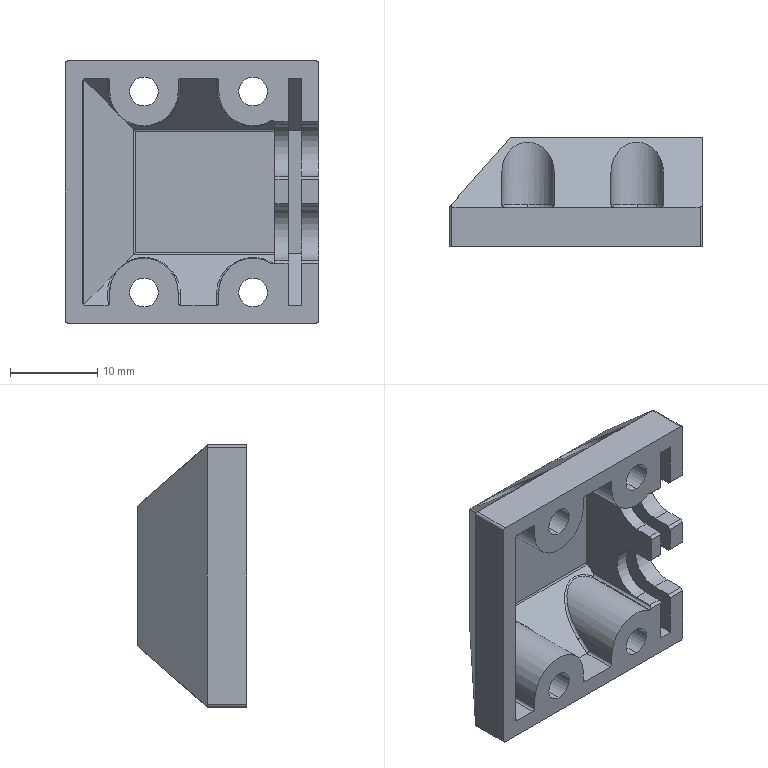Part | NX | features BREP 1 | 1 solid | 131 faces | box 29 x 12.5 x 30 mm | volume 3591 mm3 | plane 64 | cylinder 55 | torus 8 | spline 4 | commonest cylinder face diameters 0.6 x31 3.3 x8 6 x8 7.85 x6 6.2 x2